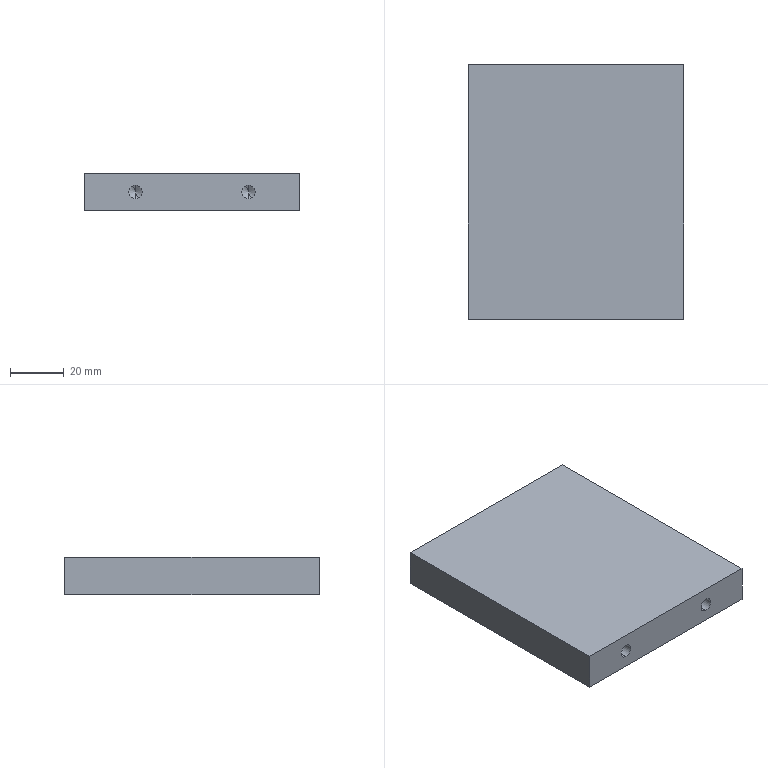Part | SolidWorks | features HoleWzd 2, Extrusion 1 | 1 solid | 22 faces | box 80 x 94.5 x 14 mm | volume 104465 mm3 | cylinder 8 | cone 8 | plane 6 | commonest cylinder face diameters 5 x8
STEP:
#1=CARTESIAN_POINT('',(33.,30.25,4.5));
#2=VERTEX_POINT('',#1);
#3=CARTESIAN_POINT('',(33.,30.25,9.5));
#4=VERTEX_POINT('',#3);
#5=CARTESIAN_POINT('',(33.,30.25,7.));
#6=DIRECTION('',(0.,1.,0.));
#7=DIRECTION('',(0.,0.,1.));
#8=AXIS2_PLACEMENT_3D('',#5,#6,#7);
#9=CIRCLE('',#8,2.5);
#10=EDGE_CURVE('',#2,#4,#9,.T.);
#11=ORIENTED_EDGE('',*,*,#10,.F.);
#12=CARTESIAN_POINT('',(33.,47.25,4.5));
#13=VERTEX_POINT('',#12);
#14=CARTESIAN_POINT('',(33.,47.25,4.5));
#15=DIRECTION('',(0.,1.,0.));
#16=VECTOR('',#15,1000.);
#17=LINE('',#14,#16);
#18=EDGE_CURVE('',#2,#13,#17,.T.);
#19=ORIENTED_EDGE('',*,*,#18,.T.);
#20=CARTESIAN_POINT('',(33.,47.25,9.5));
#21=VERTEX_POINT('',#20);
#22=CARTESIAN_POINT('',(33.,47.25,7.));
#23=DIRECTION('',(0.,1.,0.));
#24=DIRECTION('',(0.,0.,1.));
#25=AXIS2_PLACEMENT_3D('',#22,#23,#24);
#26=CIRCLE('',#25,2.5);
#27=EDGE_CURVE('',#13,#21,#26,.T.);
#28=ORIENTED_EDGE('',*,*,#27,.T.);
#29=CARTESIAN_POINT('',(33.,47.25,9.5));
#30=DIRECTION('',(0.,1.,0.));
#31=VECTOR('',#30,1000.);
#32=LINE('',#29,#31);
#33=EDGE_CURVE('',#4,#21,#32,.T.);
#34=ORIENTED_EDGE('',*,*,#33,.F.);
#35=EDGE_LOOP('',(#11,#19,#28,#34));
#36=FACE_OUTER_BOUND('',#35,.T.);
#37=CARTESIAN_POINT('',(33.,47.25,7.));
#38=DIRECTION('',(0.,1.,0.));
#39=DIRECTION('',(0.,0.,1.));
#40=AXIS2_PLACEMENT_3D('',#37,#38,#39);
#41=CYLINDRICAL_SURFACE('',#40,2.5);
#42=ADVANCED_FACE('',(#36),#41,.F.);
#43=CARTESIAN_POINT('',(33.,28.748,7.));
#44=VERTEX_POINT('',#43);
#45=CARTESIAN_POINT('',(33.,30.25,9.5));
#46=DIRECTION('',(0.,0.515,0.8572));
#47=VECTOR('',#46,1000.);
#48=LINE('',#45,#47);
#49=EDGE_CURVE('',#44,#4,#48,.T.);
#50=ORIENTED_EDGE('',*,*,#49,.F.);
#51=CARTESIAN_POINT('',(33.,30.25,4.5));
#52=DIRECTION('',(0.,0.515,-0.8572));
#53=VECTOR('',#52,1000.);
#54=LINE('',#51,#53);
#55=EDGE_CURVE('',#44,#2,#54,.T.);
#56=ORIENTED_EDGE('',*,*,#55,.T.);
#57=ORIENTED_EDGE('',*,*,#10,.T.);
#58=EDGE_LOOP('',(#50,#56,#57));
#59=FACE_OUTER_BOUND('',#58,.T.);
#60=CARTESIAN_POINT('',(33.,30.25,7.));
#61=DIRECTION('',(0.,1.,0.));
#62=DIRECTION('',(0.,0.,1.));
#63=AXIS2_PLACEMENT_3D('',#60,#61,#62);
#64=CONICAL_SURFACE('',#63,2.5,1.03);
#65=ADVANCED_FACE('',(#59),#64,.F.);
#66=CARTESIAN_POINT('',(-33.,30.25,4.5));
#67=VERTEX_POINT('',#66);
#68=CARTESIAN_POINT('',(-33.,30.25,9.5));
#69=VERTEX_POINT('',#68);
#70=CARTESIAN_POINT('',(-33.,30.25,7.));
#71=DIRECTION('',(0.,1.,0.));
#72=DIRECTION('',(0.,0.,1.));
#73=AXIS2_PLACEMENT_3D('',#70,#71,#72);
#74=CIRCLE('',#73,2.5);
#75=EDGE_CURVE('',#67,#69,#74,.T.);
#76=ORIENTED_EDGE('',*,*,#75,.F.);
#77=CARTESIAN_POINT('',(-33.,47.25,4.5));
#78=VERTEX_POINT('',#77);
#79=CARTESIAN_POINT('',(-33.,47.25,4.5));
#80=DIRECTION('',(0.,1.,0.));
#81=VECTOR('',#80,1000.);
#82=LINE('',#79,#81);
#83=EDGE_CURVE('',#67,#78,#82,.T.);
#84=ORIENTED_EDGE('',*,*,#83,.T.);
#85=CARTESIAN_POINT('',(-33.,47.25,9.5));
#86=VERTEX_POINT('',#85);
#87=CARTESIAN_POINT('',(-33.,47.25,7.));
#88=DIRECTION('',(0.,1.,0.));
#89=DIRECTION('',(0.,0.,1.));
#90=AXIS2_PLACEMENT_3D('',#87,#88,#89);
#91=CIRCLE('',#90,2.5);
#92=EDGE_CURVE('',#78,#86,#91,.T.);
#93=ORIENTED_EDGE('',*,*,#92,.T.);
#94=CARTESIAN_POINT('',(-33.,47.25,9.5));
#95=DIRECTION('',(0.,1.,0.));
#96=VECTOR('',#95,1000.);
#97=LINE('',#94,#96);
#98=EDGE_CURVE('',#69,#86,#97,.T.);
#99=ORIENTED_EDGE('',*,*,#98,.F.);
#100=EDGE_LOOP('',(#76,#84,#93,#99));
#101=FACE_OUTER_BOUND('',#100,.T.);
#102=CARTESIAN_POINT('',(-33.,47.25,7.));
#103=DIRECTION('',(0.,1.,0.));
#104=DIRECTION('',(0.,0.,1.));
#105=AXIS2_PLACEMENT_3D('',#102,#103,#104);
#106=CYLINDRICAL_SURFACE('',#105,2.5);
#107=ADVANCED_FACE('',(#101),#106,.F.);
#108=CARTESIAN_POINT('',(-33.,28.748,7.));
#109=VERTEX_POINT('',#108);
#110=CARTESIAN_POINT('',(-33.,30.25,9.5));
#111=DIRECTION('',(0.,0.515,0.8572));
#112=VECTOR('',#111,1000.);
#113=LINE('',#110,#112);
#114=EDGE_CURVE('',#109,#69,#113,.T.);
#115=ORIENTED_EDGE('',*,*,#114,.F.);
#116=CARTESIAN_POINT('',(-33.,30.25,4.5));
#117=DIRECTION('',(0.,0.515,-0.8572));
#118=VECTOR('',#117,1000.);
#119=LINE('',#116,#118);
#120=EDGE_CURVE('',#109,#67,#119,.T.);
#121=ORIENTED_EDGE('',*,*,#120,.T.);
#122=ORIENTED_EDGE('',*,*,#75,.T.);
#123=EDGE_LOOP('',(#115,#121,#122));
#124=FACE_OUTER_BOUND('',#123,.T.);
#125=CARTESIAN_POINT('',(-33.,30.25,7.));
#126=DIRECTION('',(0.,1.,0.));
#127=DIRECTION('',(0.,0.,1.));
#128=AXIS2_PLACEMENT_3D('',#125,#126,#127);
#129=CONICAL_SURFACE('',#128,2.5,1.03);
#130=ADVANCED_FACE('',(#124),#129,.F.);
#131=CARTESIAN_POINT('',(21.,-30.25,9.5));
#132=VERTEX_POINT('',#131);
#133=CARTESIAN_POINT('',(21.,-30.25,4.5));
#134=VERTEX_POINT('',#133);
#135=CARTESIAN_POINT('',(21.,-30.25,7.));
#136=DIRECTION('',(0.,-1.,0.));
#137=DIRECTION('',(0.,0.,-1.));
#138=AXIS2_PLACEMENT_3D('',#135,#136,#137);
#139=CIRCLE('',#138,2.5);
#140=EDGE_CURVE('',#132,#134,#139,.T.);
#141=ORIENTED_EDGE('',*,*,#140,.F.);
#142=CARTESIAN_POINT('',(21.,-47.25,9.5));
#143=VERTEX_POINT('',#142);
#144=CARTESIAN_POINT('',(21.,-47.25,9.5));
#145=DIRECTION('',(0.,-1.,0.));
#146=VECTOR('',#145,1000.);
#147=LINE('',#144,#146);
#148=EDGE_CURVE('',#132,#143,#147,.T.);
#149=ORIENTED_EDGE('',*,*,#148,.T.);
#150=CARTESIAN_POINT('',(21.,-47.25,4.5));
#151=VERTEX_POINT('',#150);
#152=CARTESIAN_POINT('',(21.,-47.25,7.));
#153=DIRECTION('',(0.,-1.,0.));
#154=DIRECTION('',(0.,0.,-1.));
#155=AXIS2_PLACEMENT_3D('',#152,#153,#154);
#156=CIRCLE('',#155,2.5);
#157=EDGE_CURVE('',#143,#151,#156,.T.);
#158=ORIENTED_EDGE('',*,*,#157,.T.);
#159=CARTESIAN_POINT('',(21.,-47.25,4.5));
#160=DIRECTION('',(0.,-1.,0.));
#161=VECTOR('',#160,1000.);
#162=LINE('',#159,#161);
#163=EDGE_CURVE('',#134,#151,#162,.T.);
#164=ORIENTED_EDGE('',*,*,#163,.F.);
#165=EDGE_LOOP('',(#141,#149,#158,#164));
#166=FACE_OUTER_BOUND('',#165,.T.);
#167=CARTESIAN_POINT('',(21.,-47.25,7.));
#168=DIRECTION('',(0.,-1.,0.));
#169=DIRECTION('',(0.,0.,-1.));
#170=AXIS2_PLACEMENT_3D('',#167,#168,#169);
#171=CYLINDRICAL_SURFACE('',#170,2.5);
#172=ADVANCED_FACE('',(#166),#171,.F.);
#173=CARTESIAN_POINT('',(21.,-28.748,7.));
#174=VERTEX_POINT('',#173);
#175=CARTESIAN_POINT('',(21.,-30.25,4.5));
#176=DIRECTION('',(0.,-0.515,-0.8572));
#177=VECTOR('',#176,1000.);
#178=LINE('',#175,#177);
#179=EDGE_CURVE('',#174,#134,#178,.T.);
#180=ORIENTED_EDGE('',*,*,#179,.F.);
#181=CARTESIAN_POINT('',(21.,-30.25,9.5));
#182=DIRECTION('',(0.,-0.515,0.8572));
#183=VECTOR('',#182,1000.);
#184=LINE('',#181,#183);
#185=EDGE_CURVE('',#174,#132,#184,.T.);
#186=ORIENTED_EDGE('',*,*,#185,.T.);
#187=ORIENTED_EDGE('',*,*,#140,.T.);
#188=EDGE_LOOP('',(#180,#186,#187));
#189=FACE_OUTER_BOUND('',#188,.T.);
#190=CARTESIAN_POINT('',(21.,-30.25,7.));
#191=DIRECTION('',(0.,-1.,0.));
#192=DIRECTION('',(0.,0.,-1.));
#193=AXIS2_PLACEMENT_3D('',#190,#191,#192);
#194=CONICAL_SURFACE('',#193,2.5,1.03);
#195=ADVANCED_FACE('',(#189),#194,.F.);
#196=CARTESIAN_POINT('',(-21.,-30.25,9.5));
#197=VERTEX_POINT('',#196);
#198=CARTESIAN_POINT('',(-21.,-30.25,4.5));
#199=VERTEX_POINT('',#198);
#200=CARTESIAN_POINT('',(-21.,-30.25,7.));
#201=DIRECTION('',(0.,-1.,0.));
#202=DIRECTION('',(0.,0.,-1.));
#203=AXIS2_PLACEMENT_3D('',#200,#201,#202);
#204=CIRCLE('',#203,2.5);
#205=EDGE_CURVE('',#197,#199,#204,.T.);
#206=ORIENTED_EDGE('',*,*,#205,.F.);
#207=CARTESIAN_POINT('',(-21.,-47.25,9.5));
#208=VERTEX_POINT('',#207);
#209=CARTESIAN_POINT('',(-21.,-47.25,9.5));
#210=DIRECTION('',(0.,-1.,0.));
#211=VECTOR('',#210,1000.);
#212=LINE('',#209,#211);
#213=EDGE_CURVE('',#197,#208,#212,.T.);
#214=ORIENTED_EDGE('',*,*,#213,.T.);
#215=CARTESIAN_POINT('',(-21.,-47.25,4.5));
#216=VERTEX_POINT('',#215);
#217=CARTESIAN_POINT('',(-21.,-47.25,7.));
#218=DIRECTION('',(0.,-1.,0.));
#219=DIRECTION('',(0.,0.,-1.));
#220=AXIS2_PLACEMENT_3D('',#217,#218,#219);
#221=CIRCLE('',#220,2.5);
#222=EDGE_CURVE('',#208,#216,#221,.T.);
#223=ORIENTED_EDGE('',*,*,#222,.T.);
#224=CARTESIAN_POINT('',(-21.,-47.25,4.5));
#225=DIRECTION('',(0.,-1.,0.));
#226=VECTOR('',#225,1000.);
#227=LINE('',#224,#226);
#228=EDGE_CURVE('',#199,#216,#227,.T.);
#229=ORIENTED_EDGE('',*,*,#228,.F.);
#230=EDGE_LOOP('',(#206,#214,#223,#229));
#231=FACE_OUTER_BOUND('',#230,.T.);
#232=CARTESIAN_POINT('',(-21.,-47.25,7.));
#233=DIRECTION('',(0.,-1.,0.));
#234=DIRECTION('',(0.,0.,-1.));
#235=AXIS2_PLACEMENT_3D('',#232,#233,#234);
#236=CYLINDRICAL_SURFACE('',#235,2.5);
#237=ADVANCED_FACE('',(#231),#236,.F.);
#238=CARTESIAN_POINT('',(-21.,-28.748,7.));
#239=VERTEX_POINT('',#238);
#240=CARTESIAN_POINT('',(-21.,-30.25,4.5));
#241=DIRECTION('',(0.,-0.515,-0.8572));
#242=VECTOR('',#241,1000.);
#243=LINE('',#240,#242);
#244=EDGE_CURVE('',#239,#199,#243,.T.);
#245=ORIENTED_EDGE('',*,*,#244,.F.);
#246=CARTESIAN_POINT('',(-21.,-30.25,9.5));
#247=DIRECTION('',(0.,-0.515,0.8572));
#248=VECTOR('',#247,1000.);
#249=LINE('',#246,#248);
#250=EDGE_CURVE('',#239,#197,#249,.T.);
#251=ORIENTED_EDGE('',*,*,#250,.T.);
#252=ORIENTED_EDGE('',*,*,#205,.T.);
#253=EDGE_LOOP('',(#245,#251,#252));
#254=FACE_OUTER_BOUND('',#253,.T.);
#255=CARTESIAN_POINT('',(-21.,-30.25,7.));
#256=DIRECTION('',(0.,-1.,0.));
#257=DIRECTION('',(0.,0.,-1.));
#258=AXIS2_PLACEMENT_3D('',#255,#256,#257);
#259=CONICAL_SURFACE('',#258,2.5,1.03);
#260=ADVANCED_FACE('',(#254),#259,.F.);
#261=CARTESIAN_POINT('',(40.,-47.25,0.));
#262=VERTEX_POINT('',#261);
#263=CARTESIAN_POINT('',(40.,47.25,0.));
#264=VERTEX_POINT('',#263);
#265=CARTESIAN_POINT('',(40.,47.25,0.));
#266=DIRECTION('',(0.,1.,0.));
#267=VECTOR('',#266,1000.);
#268=LINE('',#265,#267);
#269=EDGE_CURVE('',#262,#264,#268,.T.);
#270=ORIENTED_EDGE('',*,*,#269,.T.);
#271=CARTESIAN_POINT('',(40.,47.25,14.));
#272=VERTEX_POINT('',#271);
#273=CARTESIAN_POINT('',(40.,47.25,14.));
#274=DIRECTION('',(0.,0.,-1.));
#275=VECTOR('',#274,1000.);
#276=LINE('',#273,#275);
#277=EDGE_CURVE('',#272,#264,#276,.T.);
#278=ORIENTED_EDGE('',*,*,#277,.F.);
#279=CARTESIAN_POINT('',(40.,-47.25,14.));
#280=VERTEX_POINT('',#279);
#281=CARTESIAN_POINT('',(40.,47.25,14.));
#282=DIRECTION('',(0.,1.,0.));
#283=VECTOR('',#282,1000.);
#284=LINE('',#281,#283);
#285=EDGE_CURVE('',#280,#272,#284,.T.);
#286=ORIENTED_EDGE('',*,*,#285,.F.);
#287=CARTESIAN_POINT('',(40.,-47.25,14.));
#288=DIRECTION('',(0.,0.,-1.));
#289=VECTOR('',#288,1000.);
#290=LINE('',#287,#289);
#291=EDGE_CURVE('',#280,#262,#290,.T.);
#292=ORIENTED_EDGE('',*,*,#291,.T.);
#293=EDGE_LOOP('',(#270,#278,#286,#292));
#294=FACE_OUTER_BOUND('',#293,.T.);
#295=CARTESIAN_POINT('',(40.,47.25,14.));
#296=DIRECTION('',(-1.,0.,0.));
#297=DIRECTION('',(0.,-1.,0.));
#298=AXIS2_PLACEMENT_3D('',#295,#296,#297);
#299=PLANE('',#298);
#300=ADVANCED_FACE('',(#294),#299,.F.);
#301=CARTESIAN_POINT('',(33.,47.25,7.));
#302=DIRECTION('',(0.,1.,0.));
#303=DIRECTION('',(0.,0.,1.));
#304=AXIS2_PLACEMENT_3D('',#301,#302,#303);
#305=CIRCLE('',#304,2.5);
#306=EDGE_CURVE('',#21,#13,#305,.T.);
#307=ORIENTED_EDGE('',*,*,#306,.F.);
#308=ORIENTED_EDGE('',*,*,#27,.F.);
#309=EDGE_LOOP('',(#307,#308));
#310=FACE_BOUND('',#309,.T.);
#311=CARTESIAN_POINT('',(-33.,47.25,7.));
#312=DIRECTION('',(0.,1.,0.));
#313=DIRECTION('',(0.,0.,1.));
#314=AXIS2_PLACEMENT_3D('',#311,#312,#313);
#315=CIRCLE('',#314,2.5);
#316=EDGE_CURVE('',#86,#78,#315,.T.);
#317=ORIENTED_EDGE('',*,*,#316,.F.);
#318=ORIENTED_EDGE('',*,*,#92,.F.);
#319=EDGE_LOOP('',(#317,#318));
#320=FACE_BOUND('',#319,.T.);
#321=CARTESIAN_POINT('',(-40.,47.25,0.));
#322=VERTEX_POINT('',#321);
#323=CARTESIAN_POINT('',(-40.,47.25,0.));
#324=DIRECTION('',(-1.,0.,0.));
#325=VECTOR('',#324,1000.);
#326=LINE('',#323,#325);
#327=EDGE_CURVE('',#264,#322,#326,.T.);
#328=ORIENTED_EDGE('',*,*,#327,.T.);
#329=CARTESIAN_POINT('',(-40.,47.25,14.));
#330=VERTEX_POINT('',#329);
#331=CARTESIAN_POINT('',(-40.,47.25,14.));
#332=DIRECTION('',(0.,0.,-1.));
#333=VECTOR('',#332,1000.);
#334=LINE('',#331,#333);
#335=EDGE_CURVE('',#330,#322,#334,.T.);
#336=ORIENTED_EDGE('',*,*,#335,.F.);
#337=CARTESIAN_POINT('',(-40.,47.25,14.));
#338=DIRECTION('',(-1.,0.,0.));
#339=VECTOR('',#338,1000.);
#340=LINE('',#337,#339);
#341=EDGE_CURVE('',#272,#330,#340,.T.);
#342=ORIENTED_EDGE('',*,*,#341,.F.);
#343=ORIENTED_EDGE('',*,*,#277,.T.);
#344=EDGE_LOOP('',(#328,#336,#342,#343));
#345=FACE_OUTER_BOUND('',#344,.T.);
#346=CARTESIAN_POINT('',(-40.,47.25,14.));
#347=DIRECTION('',(0.,-1.,0.));
#348=DIRECTION('',(0.,0.,-1.));
#349=AXIS2_PLACEMENT_3D('',#346,#347,#348);
#350=PLANE('',#349);
#351=ADVANCED_FACE('',(#310,#320,#345),#350,.F.);
#352=CARTESIAN_POINT('',(-40.,-47.25,0.));
#353=VERTEX_POINT('',#352);
#354=CARTESIAN_POINT('',(-40.,47.25,0.));
#355=DIRECTION('',(0.,-1.,0.));
#356=VECTOR('',#355,1000.);
#357=LINE('',#354,#356);
#358=EDGE_CURVE('',#322,#353,#357,.T.);
#359=ORIENTED_EDGE('',*,*,#358,.T.);
#360=CARTESIAN_POINT('',(-40.,-47.25,14.));
#361=VERTEX_POINT('',#360);
#362=CARTESIAN_POINT('',(-40.,-47.25,14.));
#363=DIRECTION('',(0.,0.,-1.));
#364=VECTOR('',#363,1000.);
#365=LINE('',#362,#364);
#366=EDGE_CURVE('',#361,#353,#365,.T.);
#367=ORIENTED_EDGE('',*,*,#366,.F.);
#368=CARTESIAN_POINT('',(-40.,47.25,14.));
#369=DIRECTION('',(0.,-1.,0.));
#370=VECTOR('',#369,1000.);
#371=LINE('',#368,#370);
#372=EDGE_CURVE('',#330,#361,#371,.T.);
#373=ORIENTED_EDGE('',*,*,#372,.F.);
#374=ORIENTED_EDGE('',*,*,#335,.T.);
#375=EDGE_LOOP('',(#359,#367,#373,#374));
#376=FACE_OUTER_BOUND('',#375,.T.);
#377=CARTESIAN_POINT('',(-40.,47.25,14.));
#378=DIRECTION('',(1.,0.,0.));
#379=DIRECTION('',(0.,1.,0.));
#380=AXIS2_PLACEMENT_3D('',#377,#378,#379);
#381=PLANE('',#380);
#382=ADVANCED_FACE('',(#376),#381,.F.);
#383=CARTESIAN_POINT('',(21.,-47.25,7.));
#384=DIRECTION('',(0.,-1.,0.));
#385=DIRECTION('',(0.,0.,-1.));
#386=AXIS2_PLACEMENT_3D('',#383,#384,#385);
#387=CIRCLE('',#386,2.5);
#388=EDGE_CURVE('',#151,#143,#387,.T.);
#389=ORIENTED_EDGE('',*,*,#388,.F.);
#390=ORIENTED_EDGE('',*,*,#157,.F.);
#391=EDGE_LOOP('',(#389,#390));
#392=FACE_BOUND('',#391,.T.);
#393=CARTESIAN_POINT('',(-21.,-47.25,7.));
#394=DIRECTION('',(0.,-1.,0.));
#395=DIRECTION('',(0.,0.,-1.));
#396=AXIS2_PLACEMENT_3D('',#393,#394,#395);
#397=CIRCLE('',#396,2.5);
#398=EDGE_CURVE('',#216,#208,#397,.T.);
#399=ORIENTED_EDGE('',*,*,#398,.F.);
#400=ORIENTED_EDGE('',*,*,#222,.F.);
#401=EDGE_LOOP('',(#399,#400));
#402=FACE_BOUND('',#401,.T.);
#403=CARTESIAN_POINT('',(-40.,-47.25,0.));
#404=DIRECTION('',(1.,0.,0.));
#405=VECTOR('',#404,1000.);
#406=LINE('',#403,#405);
#407=EDGE_CURVE('',#353,#262,#406,.T.);
#408=ORIENTED_EDGE('',*,*,#407,.T.);
#409=ORIENTED_EDGE('',*,*,#291,.F.);
#410=CARTESIAN_POINT('',(-40.,-47.25,14.));
#411=DIRECTION('',(1.,0.,0.));
#412=VECTOR('',#411,1000.);
#413=LINE('',#410,#412);
#414=EDGE_CURVE('',#361,#280,#413,.T.);
#415=ORIENTED_EDGE('',*,*,#414,.F.);
#416=ORIENTED_EDGE('',*,*,#366,.T.);
#417=EDGE_LOOP('',(#408,#409,#415,#416));
#418=FACE_OUTER_BOUND('',#417,.T.);
#419=CARTESIAN_POINT('',(-40.,-47.25,14.));
#420=DIRECTION('',(0.,1.,0.));
#421=DIRECTION('',(0.,0.,1.));
#422=AXIS2_PLACEMENT_3D('',#419,#420,#421);
#423=PLANE('',#422);
#424=ADVANCED_FACE('',(#392,#402,#418),#423,.F.);
#425=ORIENTED_EDGE('',*,*,#285,.T.);
#426=ORIENTED_EDGE('',*,*,#341,.T.);
#427=ORIENTED_EDGE('',*,*,#372,.T.);
#428=ORIENTED_EDGE('',*,*,#414,.T.);
#429=EDGE_LOOP('',(#425,#426,#427,#428));
#430=FACE_OUTER_BOUND('',#429,.T.);
#431=CARTESIAN_POINT('',(0.,0.,14.));
#432=DIRECTION('',(0.,0.,1.));
#433=DIRECTION('',(1.,0.,0.));
#434=AXIS2_PLACEMENT_3D('',#431,#432,#433);
#435=PLANE('',#434);
#436=ADVANCED_FACE('',(#430),#435,.T.);
#437=ORIENTED_EDGE('',*,*,#269,.F.);
#438=ORIENTED_EDGE('',*,*,#407,.F.);
#439=ORIENTED_EDGE('',*,*,#358,.F.);
#440=ORIENTED_EDGE('',*,*,#327,.F.);
#441=EDGE_LOOP('',(#437,#438,#439,#440));
#442=FACE_OUTER_BOUND('',#441,.T.);
#443=CARTESIAN_POINT('',(0.,0.,0.));
#444=DIRECTION('',(0.,0.,1.));
#445=DIRECTION('',(1.,0.,0.));
#446=AXIS2_PLACEMENT_3D('',#443,#444,#445);
#447=PLANE('',#446);
#448=ADVANCED_FACE('',(#442),#447,.F.);
#449=ORIENTED_EDGE('',*,*,#250,.F.);
#450=ORIENTED_EDGE('',*,*,#244,.T.);
#451=CARTESIAN_POINT('',(-21.,-30.25,7.));
#452=DIRECTION('',(0.,-1.,0.));
#453=DIRECTION('',(0.,0.,-1.));
#454=AXIS2_PLACEMENT_3D('',#451,#452,#453);
#455=CIRCLE('',#454,2.5);
#456=EDGE_CURVE('',#199,#197,#455,.T.);
#457=ORIENTED_EDGE('',*,*,#456,.T.);
#458=EDGE_LOOP('',(#449,#450,#457));
#459=FACE_OUTER_BOUND('',#458,.T.);
#460=CARTESIAN_POINT('',(-21.,-30.25,7.));
#461=DIRECTION('',(0.,-1.,0.));
#462=DIRECTION('',(0.,0.,-1.));
#463=AXIS2_PLACEMENT_3D('',#460,#461,#462);
#464=CONICAL_SURFACE('',#463,2.5,1.03);
#465=ADVANCED_FACE('',(#459),#464,.F.);
#466=ORIENTED_EDGE('',*,*,#213,.F.);
#467=ORIENTED_EDGE('',*,*,#456,.F.);
#468=ORIENTED_EDGE('',*,*,#228,.T.);
#469=ORIENTED_EDGE('',*,*,#398,.T.);
#470=EDGE_LOOP('',(#466,#467,#468,#469));
#471=FACE_OUTER_BOUND('',#470,.T.);
#472=CARTESIAN_POINT('',(-21.,-47.25,7.));
#473=DIRECTION('',(0.,-1.,0.));
#474=DIRECTION('',(0.,0.,-1.));
#475=AXIS2_PLACEMENT_3D('',#472,#473,#474);
#476=CYLINDRICAL_SURFACE('',#475,2.5);
#477=ADVANCED_FACE('',(#471),#476,.F.);
#478=ORIENTED_EDGE('',*,*,#185,.F.);
#479=ORIENTED_EDGE('',*,*,#179,.T.);
#480=CARTESIAN_POINT('',(21.,-30.25,7.));
#481=DIRECTION('',(0.,-1.,0.));
#482=DIRECTION('',(0.,0.,-1.));
#483=AXIS2_PLACEMENT_3D('',#480,#481,#482);
#484=CIRCLE('',#483,2.5);
#485=EDGE_CURVE('',#134,#132,#484,.T.);
#486=ORIENTED_EDGE('',*,*,#485,.T.);
#487=EDGE_LOOP('',(#478,#479,#486));
#488=FACE_OUTER_BOUND('',#487,.T.);
#489=CARTESIAN_POINT('',(21.,-30.25,7.));
#490=DIRECTION('',(0.,-1.,0.));
#491=DIRECTION('',(0.,0.,-1.));
#492=AXIS2_PLACEMENT_3D('',#489,#490,#491);
#493=CONICAL_SURFACE('',#492,2.5,1.03);
#494=ADVANCED_FACE('',(#488),#493,.F.);
#495=ORIENTED_EDGE('',*,*,#148,.F.);
#496=ORIENTED_EDGE('',*,*,#485,.F.);
#497=ORIENTED_EDGE('',*,*,#163,.T.);
#498=ORIENTED_EDGE('',*,*,#388,.T.);
#499=EDGE_LOOP('',(#495,#496,#497,#498));
#500=FACE_OUTER_BOUND('',#499,.T.);
#501=CARTESIAN_POINT('',(21.,-47.25,7.));
#502=DIRECTION('',(0.,-1.,0.));
#503=DIRECTION('',(0.,0.,-1.));
#504=AXIS2_PLACEMENT_3D('',#501,#502,#503);
#505=CYLINDRICAL_SURFACE('',#504,2.5);
#506=ADVANCED_FACE('',(#500),#505,.F.);
#507=ORIENTED_EDGE('',*,*,#120,.F.);
#508=ORIENTED_EDGE('',*,*,#114,.T.);
#509=CARTESIAN_POINT('',(-33.,30.25,7.));
#510=DIRECTION('',(0.,1.,0.));
#511=DIRECTION('',(0.,0.,1.));
#512=AXIS2_PLACEMENT_3D('',#509,#510,#511);
#513=CIRCLE('',#512,2.5);
#514=EDGE_CURVE('',#69,#67,#513,.T.);
#515=ORIENTED_EDGE('',*,*,#514,.T.);
#516=EDGE_LOOP('',(#507,#508,#515));
#517=FACE_OUTER_BOUND('',#516,.T.);
#518=CARTESIAN_POINT('',(-33.,30.25,7.));
#519=DIRECTION('',(0.,1.,0.));
#520=DIRECTION('',(0.,0.,1.));
#521=AXIS2_PLACEMENT_3D('',#518,#519,#520);
#522=CONICAL_SURFACE('',#521,2.5,1.03);
#523=ADVANCED_FACE('',(#517),#522,.F.);
#524=ORIENTED_EDGE('',*,*,#83,.F.);
#525=ORIENTED_EDGE('',*,*,#514,.F.);
#526=ORIENTED_EDGE('',*,*,#98,.T.);
#527=ORIENTED_EDGE('',*,*,#316,.T.);
#528=EDGE_LOOP('',(#524,#525,#526,#527));
#529=FACE_OUTER_BOUND('',#528,.T.);
#530=CARTESIAN_POINT('',(-33.,47.25,7.));
#531=DIRECTION('',(0.,1.,0.));
#532=DIRECTION('',(0.,0.,1.));
#533=AXIS2_PLACEMENT_3D('',#530,#531,#532);
#534=CYLINDRICAL_SURFACE('',#533,2.5);
#535=ADVANCED_FACE('',(#529),#534,.F.);
#536=ORIENTED_EDGE('',*,*,#55,.F.);
#537=ORIENTED_EDGE('',*,*,#49,.T.);
#538=CARTESIAN_POINT('',(33.,30.25,7.));
#539=DIRECTION('',(0.,1.,0.));
#540=DIRECTION('',(0.,0.,1.));
#541=AXIS2_PLACEMENT_3D('',#538,#539,#540);
#542=CIRCLE('',#541,2.5);
#543=EDGE_CURVE('',#4,#2,#542,.T.);
#544=ORIENTED_EDGE('',*,*,#543,.T.);
#545=EDGE_LOOP('',(#536,#537,#544));
#546=FACE_OUTER_BOUND('',#545,.T.);
#547=CARTESIAN_POINT('',(33.,30.25,7.));
#548=DIRECTION('',(0.,1.,0.));
#549=DIRECTION('',(0.,0.,1.));
#550=AXIS2_PLACEMENT_3D('',#547,#548,#549);
#551=CONICAL_SURFACE('',#550,2.5,1.03);
#552=ADVANCED_FACE('',(#546),#551,.F.);
#553=ORIENTED_EDGE('',*,*,#18,.F.);
#554=ORIENTED_EDGE('',*,*,#543,.F.);
#555=ORIENTED_EDGE('',*,*,#33,.T.);
#556=ORIENTED_EDGE('',*,*,#306,.T.);
#557=EDGE_LOOP('',(#553,#554,#555,#556));
#558=FACE_OUTER_BOUND('',#557,.T.);
#559=CARTESIAN_POINT('',(33.,47.25,7.));
#560=DIRECTION('',(0.,1.,0.));
#561=DIRECTION('',(0.,0.,1.));
#562=AXIS2_PLACEMENT_3D('',#559,#560,#561);
#563=CYLINDRICAL_SURFACE('',#562,2.5);
#564=ADVANCED_FACE('',(#558),#563,.F.);
#565=CLOSED_SHELL('',(#42,#65,#107,#130,#172,#195,#237,#260,#300,#351,#382,#424,#436,#448,#465,#477,#494,#506,#523,#535,#552,#564));
#566=MANIFOLD_SOLID_BREP('',#565);
#567=CARTESIAN_POINT('',(0.,0.,0.));
#568=DIRECTION('',(0.,0.,1.));
#569=DIRECTION('',(1.,0.,0.));
#570=AXIS2_PLACEMENT_3D('',#567,#568,#569);
#571=(LENGTH_UNIT()NAMED_UNIT(*)SI_UNIT(.MILLI.,.METRE.));
#572=UNCERTAINTY_MEASURE_WITH_UNIT(LENGTH_MEASURE(0.00001),#571,'','');
#573=(NAMED_UNIT(*)PLANE_ANGLE_UNIT()SI_UNIT($,.RADIAN.));
#574=(NAMED_UNIT(*)SI_UNIT($,.STERADIAN.)SOLID_ANGLE_UNIT());
#575=(GEOMETRIC_REPRESENTATION_CONTEXT(3)GLOBAL_UNCERTAINTY_ASSIGNED_CONTEXT((#572))GLOBAL_UNIT_ASSIGNED_CONTEXT((#571,#573,#574))REPRESENTATION_CONTEXT('',''));
#576=ADVANCED_BREP_SHAPE_REPRESENTATION('',(#566,#570),#575);